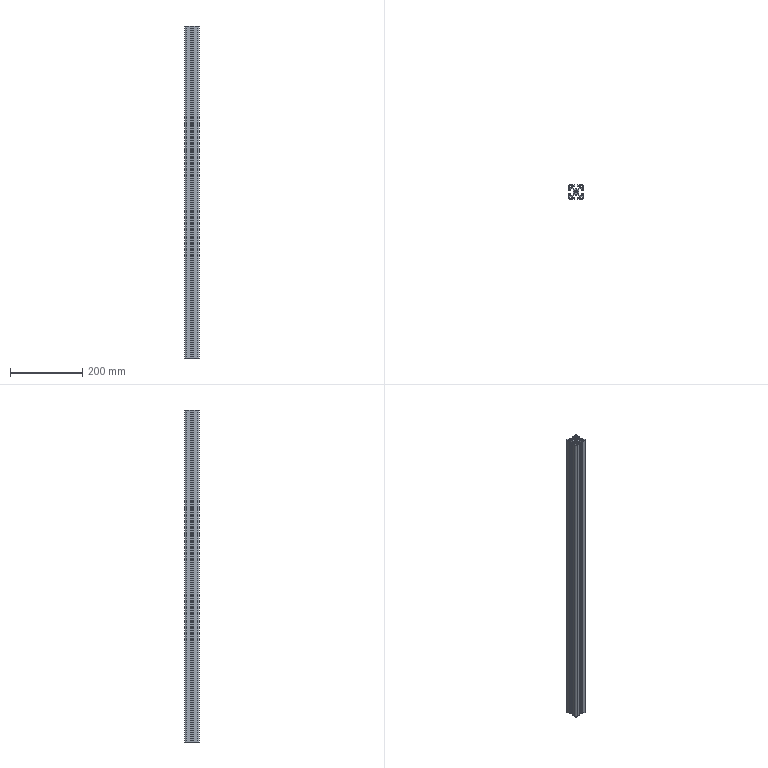Part | SolidWorks | features Extrusion 1 | 1 solid | 147 faces | box 40 x 40 x 922 mm | volume 554211 mm3 | plane 117 | cylinder 30 | commonest cylinder face diameters 1 x8 2 x8 6.8 x5 5 x4 9 x4 1.414 x1